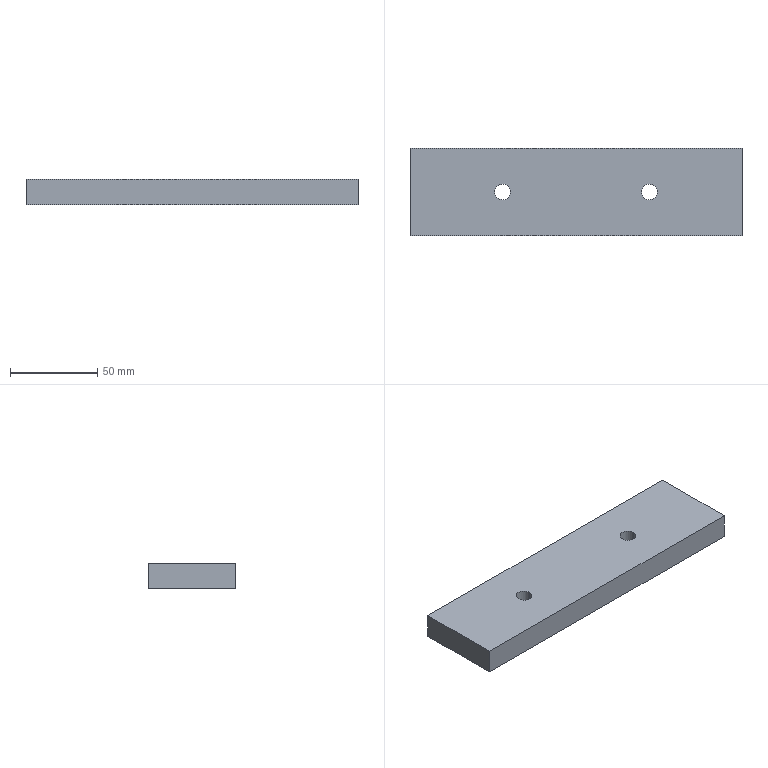Part | SolidWorks | features Extrusion 1 | 1 solid | 10 faces | box 190 x 50 x 14.5 mm | volume 135905 mm3 | plane 6 | cylinder 4 | commonest cylinder face diameters 9 x4
STEP:
#1=CARTESIAN_POINT('',(37.5,0.,7.25));
#2=VERTEX_POINT('',#1);
#3=CARTESIAN_POINT('',(46.5,0.,7.25));
#4=VERTEX_POINT('',#3);
#5=CARTESIAN_POINT('',(42.,0.,7.25));
#6=DIRECTION('',(0.,0.,1.));
#7=DIRECTION('',(1.,0.,0.));
#8=AXIS2_PLACEMENT_3D('',#5,#6,#7);
#9=CIRCLE('',#8,4.5);
#10=EDGE_CURVE('',#2,#4,#9,.T.);
#11=ORIENTED_EDGE('',*,*,#10,.T.);
#12=CARTESIAN_POINT('',(46.5,0.,-7.25));
#13=VERTEX_POINT('',#12);
#14=CARTESIAN_POINT('',(46.5,0.,7.25));
#15=DIRECTION('',(0.,0.,-1.));
#16=VECTOR('',#15,1000.);
#17=LINE('',#14,#16);
#18=EDGE_CURVE('',#4,#13,#17,.T.);
#19=ORIENTED_EDGE('',*,*,#18,.T.);
#20=CARTESIAN_POINT('',(37.5,0.,-7.25));
#21=VERTEX_POINT('',#20);
#22=CARTESIAN_POINT('',(42.,0.,-7.25));
#23=DIRECTION('',(0.,0.,1.));
#24=DIRECTION('',(1.,0.,0.));
#25=AXIS2_PLACEMENT_3D('',#22,#23,#24);
#26=CIRCLE('',#25,4.5);
#27=EDGE_CURVE('',#21,#13,#26,.T.);
#28=ORIENTED_EDGE('',*,*,#27,.F.);
#29=CARTESIAN_POINT('',(37.5,0.,7.25));
#30=DIRECTION('',(0.,0.,-1.));
#31=VECTOR('',#30,1000.);
#32=LINE('',#29,#31);
#33=EDGE_CURVE('',#2,#21,#32,.T.);
#34=ORIENTED_EDGE('',*,*,#33,.F.);
#35=EDGE_LOOP('',(#11,#19,#28,#34));
#36=FACE_OUTER_BOUND('',#35,.T.);
#37=CARTESIAN_POINT('',(42.,0.,7.25));
#38=DIRECTION('',(0.,0.,-1.));
#39=DIRECTION('',(-1.,0.,0.));
#40=AXIS2_PLACEMENT_3D('',#37,#38,#39);
#41=CYLINDRICAL_SURFACE('',#40,4.5);
#42=ADVANCED_FACE('',(#36),#41,.F.);
#43=CARTESIAN_POINT('',(-46.5,0.,7.25));
#44=VERTEX_POINT('',#43);
#45=CARTESIAN_POINT('',(-37.5,0.,7.25));
#46=VERTEX_POINT('',#45);
#47=CARTESIAN_POINT('',(-42.,0.,7.25));
#48=DIRECTION('',(0.,0.,1.));
#49=DIRECTION('',(1.,0.,0.));
#50=AXIS2_PLACEMENT_3D('',#47,#48,#49);
#51=CIRCLE('',#50,4.5);
#52=EDGE_CURVE('',#44,#46,#51,.T.);
#53=ORIENTED_EDGE('',*,*,#52,.T.);
#54=CARTESIAN_POINT('',(-37.5,0.,-7.25));
#55=VERTEX_POINT('',#54);
#56=CARTESIAN_POINT('',(-37.5,0.,7.25));
#57=DIRECTION('',(0.,0.,-1.));
#58=VECTOR('',#57,1000.);
#59=LINE('',#56,#58);
#60=EDGE_CURVE('',#46,#55,#59,.T.);
#61=ORIENTED_EDGE('',*,*,#60,.T.);
#62=CARTESIAN_POINT('',(-46.5,0.,-7.25));
#63=VERTEX_POINT('',#62);
#64=CARTESIAN_POINT('',(-42.,0.,-7.25));
#65=DIRECTION('',(0.,0.,1.));
#66=DIRECTION('',(1.,0.,0.));
#67=AXIS2_PLACEMENT_3D('',#64,#65,#66);
#68=CIRCLE('',#67,4.5);
#69=EDGE_CURVE('',#63,#55,#68,.T.);
#70=ORIENTED_EDGE('',*,*,#69,.F.);
#71=CARTESIAN_POINT('',(-46.5,0.,7.25));
#72=DIRECTION('',(0.,0.,-1.));
#73=VECTOR('',#72,1000.);
#74=LINE('',#71,#73);
#75=EDGE_CURVE('',#44,#63,#74,.T.);
#76=ORIENTED_EDGE('',*,*,#75,.F.);
#77=EDGE_LOOP('',(#53,#61,#70,#76));
#78=FACE_OUTER_BOUND('',#77,.T.);
#79=CARTESIAN_POINT('',(-42.,0.,7.25));
#80=DIRECTION('',(0.,0.,-1.));
#81=DIRECTION('',(-1.,0.,0.));
#82=AXIS2_PLACEMENT_3D('',#79,#80,#81);
#83=CYLINDRICAL_SURFACE('',#82,4.5);
#84=ADVANCED_FACE('',(#78),#83,.F.);
#85=ORIENTED_EDGE('',*,*,#52,.F.);
#86=CARTESIAN_POINT('',(-42.,0.,7.25));
#87=DIRECTION('',(0.,0.,1.));
#88=DIRECTION('',(1.,0.,0.));
#89=AXIS2_PLACEMENT_3D('',#86,#87,#88);
#90=CIRCLE('',#89,4.5);
#91=EDGE_CURVE('',#46,#44,#90,.T.);
#92=ORIENTED_EDGE('',*,*,#91,.F.);
#93=EDGE_LOOP('',(#85,#92));
#94=FACE_BOUND('',#93,.T.);
#95=CARTESIAN_POINT('',(95.,-25.,7.25));
#96=VERTEX_POINT('',#95);
#97=CARTESIAN_POINT('',(95.,25.,7.25));
#98=VERTEX_POINT('',#97);
#99=CARTESIAN_POINT('',(95.,25.,7.25));
#100=DIRECTION('',(0.,1.,0.));
#101=VECTOR('',#100,1000.);
#102=LINE('',#99,#101);
#103=EDGE_CURVE('',#96,#98,#102,.T.);
#104=ORIENTED_EDGE('',*,*,#103,.T.);
#105=CARTESIAN_POINT('',(-95.,25.,7.25));
#106=VERTEX_POINT('',#105);
#107=CARTESIAN_POINT('',(-95.,25.,7.25));
#108=DIRECTION('',(-1.,0.,0.));
#109=VECTOR('',#108,1000.);
#110=LINE('',#107,#109);
#111=EDGE_CURVE('',#98,#106,#110,.T.);
#112=ORIENTED_EDGE('',*,*,#111,.T.);
#113=CARTESIAN_POINT('',(-95.,-25.,7.25));
#114=VERTEX_POINT('',#113);
#115=CARTESIAN_POINT('',(-95.,25.,7.25));
#116=DIRECTION('',(0.,-1.,0.));
#117=VECTOR('',#116,1000.);
#118=LINE('',#115,#117);
#119=EDGE_CURVE('',#106,#114,#118,.T.);
#120=ORIENTED_EDGE('',*,*,#119,.T.);
#121=CARTESIAN_POINT('',(-95.,-25.,7.25));
#122=DIRECTION('',(1.,0.,0.));
#123=VECTOR('',#122,1000.);
#124=LINE('',#121,#123);
#125=EDGE_CURVE('',#114,#96,#124,.T.);
#126=ORIENTED_EDGE('',*,*,#125,.T.);
#127=EDGE_LOOP('',(#104,#112,#120,#126));
#128=FACE_OUTER_BOUND('',#127,.T.);
#129=ORIENTED_EDGE('',*,*,#10,.F.);
#130=CARTESIAN_POINT('',(42.,0.,7.25));
#131=DIRECTION('',(0.,0.,1.));
#132=DIRECTION('',(1.,0.,0.));
#133=AXIS2_PLACEMENT_3D('',#130,#131,#132);
#134=CIRCLE('',#133,4.5);
#135=EDGE_CURVE('',#4,#2,#134,.T.);
#136=ORIENTED_EDGE('',*,*,#135,.F.);
#137=EDGE_LOOP('',(#129,#136));
#138=FACE_BOUND('',#137,.T.);
#139=CARTESIAN_POINT('',(0.,0.,7.25));
#140=DIRECTION('',(0.,0.,1.));
#141=DIRECTION('',(1.,0.,0.));
#142=AXIS2_PLACEMENT_3D('',#139,#140,#141);
#143=PLANE('',#142);
#144=ADVANCED_FACE('',(#94,#128,#138),#143,.T.);
#145=ORIENTED_EDGE('',*,*,#69,.T.);
#146=CARTESIAN_POINT('',(-42.,0.,-7.25));
#147=DIRECTION('',(0.,0.,1.));
#148=DIRECTION('',(1.,0.,0.));
#149=AXIS2_PLACEMENT_3D('',#146,#147,#148);
#150=CIRCLE('',#149,4.5);
#151=EDGE_CURVE('',#55,#63,#150,.T.);
#152=ORIENTED_EDGE('',*,*,#151,.T.);
#153=EDGE_LOOP('',(#145,#152));
#154=FACE_BOUND('',#153,.T.);
#155=CARTESIAN_POINT('',(95.,-25.,-7.25));
#156=VERTEX_POINT('',#155);
#157=CARTESIAN_POINT('',(95.,25.,-7.25));
#158=VERTEX_POINT('',#157);
#159=CARTESIAN_POINT('',(95.,25.,-7.25));
#160=DIRECTION('',(0.,1.,0.));
#161=VECTOR('',#160,1000.);
#162=LINE('',#159,#161);
#163=EDGE_CURVE('',#156,#158,#162,.T.);
#164=ORIENTED_EDGE('',*,*,#163,.F.);
#165=CARTESIAN_POINT('',(-95.,-25.,-7.25));
#166=VERTEX_POINT('',#165);
#167=CARTESIAN_POINT('',(-95.,-25.,-7.25));
#168=DIRECTION('',(1.,0.,0.));
#169=VECTOR('',#168,1000.);
#170=LINE('',#167,#169);
#171=EDGE_CURVE('',#166,#156,#170,.T.);
#172=ORIENTED_EDGE('',*,*,#171,.F.);
#173=CARTESIAN_POINT('',(-95.,25.,-7.25));
#174=VERTEX_POINT('',#173);
#175=CARTESIAN_POINT('',(-95.,25.,-7.25));
#176=DIRECTION('',(0.,-1.,0.));
#177=VECTOR('',#176,1000.);
#178=LINE('',#175,#177);
#179=EDGE_CURVE('',#174,#166,#178,.T.);
#180=ORIENTED_EDGE('',*,*,#179,.F.);
#181=CARTESIAN_POINT('',(-95.,25.,-7.25));
#182=DIRECTION('',(-1.,0.,0.));
#183=VECTOR('',#182,1000.);
#184=LINE('',#181,#183);
#185=EDGE_CURVE('',#158,#174,#184,.T.);
#186=ORIENTED_EDGE('',*,*,#185,.F.);
#187=EDGE_LOOP('',(#164,#172,#180,#186));
#188=FACE_OUTER_BOUND('',#187,.T.);
#189=ORIENTED_EDGE('',*,*,#27,.T.);
#190=CARTESIAN_POINT('',(42.,0.,-7.25));
#191=DIRECTION('',(0.,0.,1.));
#192=DIRECTION('',(1.,0.,0.));
#193=AXIS2_PLACEMENT_3D('',#190,#191,#192);
#194=CIRCLE('',#193,4.5);
#195=EDGE_CURVE('',#13,#21,#194,.T.);
#196=ORIENTED_EDGE('',*,*,#195,.T.);
#197=EDGE_LOOP('',(#189,#196));
#198=FACE_BOUND('',#197,.T.);
#199=CARTESIAN_POINT('',(0.,0.,-7.25));
#200=DIRECTION('',(0.,0.,1.));
#201=DIRECTION('',(1.,0.,0.));
#202=AXIS2_PLACEMENT_3D('',#199,#200,#201);
#203=PLANE('',#202);
#204=ADVANCED_FACE('',(#154,#188,#198),#203,.F.);
#205=ORIENTED_EDGE('',*,*,#163,.T.);
#206=CARTESIAN_POINT('',(95.,25.,7.25));
#207=DIRECTION('',(0.,0.,-1.));
#208=VECTOR('',#207,1000.);
#209=LINE('',#206,#208);
#210=EDGE_CURVE('',#98,#158,#209,.T.);
#211=ORIENTED_EDGE('',*,*,#210,.F.);
#212=ORIENTED_EDGE('',*,*,#103,.F.);
#213=CARTESIAN_POINT('',(95.,-25.,7.25));
#214=DIRECTION('',(0.,0.,-1.));
#215=VECTOR('',#214,1000.);
#216=LINE('',#213,#215);
#217=EDGE_CURVE('',#96,#156,#216,.T.);
#218=ORIENTED_EDGE('',*,*,#217,.T.);
#219=EDGE_LOOP('',(#205,#211,#212,#218));
#220=FACE_OUTER_BOUND('',#219,.T.);
#221=CARTESIAN_POINT('',(95.,25.,7.25));
#222=DIRECTION('',(-1.,0.,0.));
#223=DIRECTION('',(0.,0.,1.));
#224=AXIS2_PLACEMENT_3D('',#221,#222,#223);
#225=PLANE('',#224);
#226=ADVANCED_FACE('',(#220),#225,.F.);
#227=ORIENTED_EDGE('',*,*,#185,.T.);
#228=CARTESIAN_POINT('',(-95.,25.,7.25));
#229=DIRECTION('',(0.,0.,-1.));
#230=VECTOR('',#229,1000.);
#231=LINE('',#228,#230);
#232=EDGE_CURVE('',#106,#174,#231,.T.);
#233=ORIENTED_EDGE('',*,*,#232,.F.);
#234=ORIENTED_EDGE('',*,*,#111,.F.);
#235=ORIENTED_EDGE('',*,*,#210,.T.);
#236=EDGE_LOOP('',(#227,#233,#234,#235));
#237=FACE_OUTER_BOUND('',#236,.T.);
#238=CARTESIAN_POINT('',(-95.,25.,7.25));
#239=DIRECTION('',(0.,-1.,0.));
#240=DIRECTION('',(0.,0.,-1.));
#241=AXIS2_PLACEMENT_3D('',#238,#239,#240);
#242=PLANE('',#241);
#243=ADVANCED_FACE('',(#237),#242,.F.);
#244=ORIENTED_EDGE('',*,*,#179,.T.);
#245=CARTESIAN_POINT('',(-95.,-25.,7.25));
#246=DIRECTION('',(0.,0.,-1.));
#247=VECTOR('',#246,1000.);
#248=LINE('',#245,#247);
#249=EDGE_CURVE('',#114,#166,#248,.T.);
#250=ORIENTED_EDGE('',*,*,#249,.F.);
#251=ORIENTED_EDGE('',*,*,#119,.F.);
#252=ORIENTED_EDGE('',*,*,#232,.T.);
#253=EDGE_LOOP('',(#244,#250,#251,#252));
#254=FACE_OUTER_BOUND('',#253,.T.);
#255=CARTESIAN_POINT('',(-95.,25.,7.25));
#256=DIRECTION('',(1.,0.,0.));
#257=DIRECTION('',(0.,0.,-1.));
#258=AXIS2_PLACEMENT_3D('',#255,#256,#257);
#259=PLANE('',#258);
#260=ADVANCED_FACE('',(#254),#259,.F.);
#261=ORIENTED_EDGE('',*,*,#171,.T.);
#262=ORIENTED_EDGE('',*,*,#217,.F.);
#263=ORIENTED_EDGE('',*,*,#125,.F.);
#264=ORIENTED_EDGE('',*,*,#249,.T.);
#265=EDGE_LOOP('',(#261,#262,#263,#264));
#266=FACE_OUTER_BOUND('',#265,.T.);
#267=CARTESIAN_POINT('',(-95.,-25.,7.25));
#268=DIRECTION('',(0.,1.,0.));
#269=DIRECTION('',(0.,0.,1.));
#270=AXIS2_PLACEMENT_3D('',#267,#268,#269);
#271=PLANE('',#270);
#272=ADVANCED_FACE('',(#266),#271,.F.);
#273=ORIENTED_EDGE('',*,*,#60,.F.);
#274=ORIENTED_EDGE('',*,*,#91,.T.);
#275=ORIENTED_EDGE('',*,*,#75,.T.);
#276=ORIENTED_EDGE('',*,*,#151,.F.);
#277=EDGE_LOOP('',(#273,#274,#275,#276));
#278=FACE_OUTER_BOUND('',#277,.T.);
#279=CARTESIAN_POINT('',(-42.,0.,7.25));
#280=DIRECTION('',(0.,0.,-1.));
#281=DIRECTION('',(-1.,0.,0.));
#282=AXIS2_PLACEMENT_3D('',#279,#280,#281);
#283=CYLINDRICAL_SURFACE('',#282,4.5);
#284=ADVANCED_FACE('',(#278),#283,.F.);
#285=ORIENTED_EDGE('',*,*,#18,.F.);
#286=ORIENTED_EDGE('',*,*,#135,.T.);
#287=ORIENTED_EDGE('',*,*,#33,.T.);
#288=ORIENTED_EDGE('',*,*,#195,.F.);
#289=EDGE_LOOP('',(#285,#286,#287,#288));
#290=FACE_OUTER_BOUND('',#289,.T.);
#291=CARTESIAN_POINT('',(42.,0.,7.25));
#292=DIRECTION('',(0.,0.,-1.));
#293=DIRECTION('',(-1.,0.,0.));
#294=AXIS2_PLACEMENT_3D('',#291,#292,#293);
#295=CYLINDRICAL_SURFACE('',#294,4.5);
#296=ADVANCED_FACE('',(#290),#295,.F.);
#297=CLOSED_SHELL('',(#42,#84,#144,#204,#226,#243,#260,#272,#284,#296));
#298=MANIFOLD_SOLID_BREP('',#297);
#299=CARTESIAN_POINT('',(0.,0.,0.));
#300=DIRECTION('',(0.,0.,1.));
#301=DIRECTION('',(1.,0.,0.));
#302=AXIS2_PLACEMENT_3D('',#299,#300,#301);
#303=(LENGTH_UNIT()NAMED_UNIT(*)SI_UNIT(.MILLI.,.METRE.));
#304=UNCERTAINTY_MEASURE_WITH_UNIT(LENGTH_MEASURE(0.00001),#303,'','');
#305=(NAMED_UNIT(*)PLANE_ANGLE_UNIT()SI_UNIT($,.RADIAN.));
#306=(NAMED_UNIT(*)SI_UNIT($,.STERADIAN.)SOLID_ANGLE_UNIT());
#307=(GEOMETRIC_REPRESENTATION_CONTEXT(3)GLOBAL_UNCERTAINTY_ASSIGNED_CONTEXT((#304))GLOBAL_UNIT_ASSIGNED_CONTEXT((#303,#305,#306))REPRESENTATION_CONTEXT('',''));
#308=ADVANCED_BREP_SHAPE_REPRESENTATION('',(#298,#302),#307);